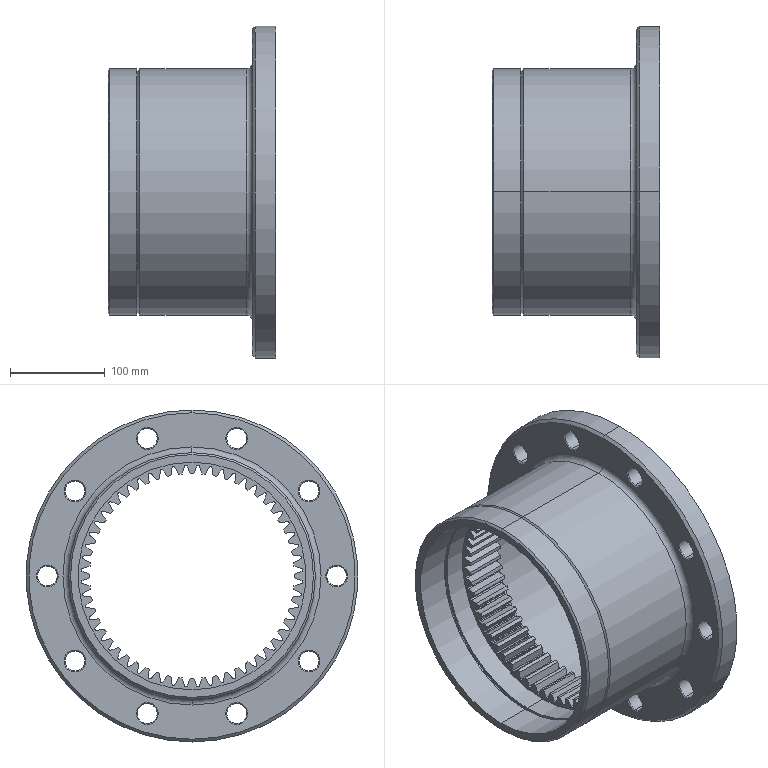Part | STEP file | Internal ring gear A m=4  Z=56 | 1 solid | 487 faces | box 177 x 350 x 350 mm | volume 2601765 mm3 | cylinder 281 | spline 112 | plane 64 | cone 26 | torus 4 | commonest cylinder face diameters 3.04 x132 216 x57 234 x56 21 x20 240 x6 260 x4